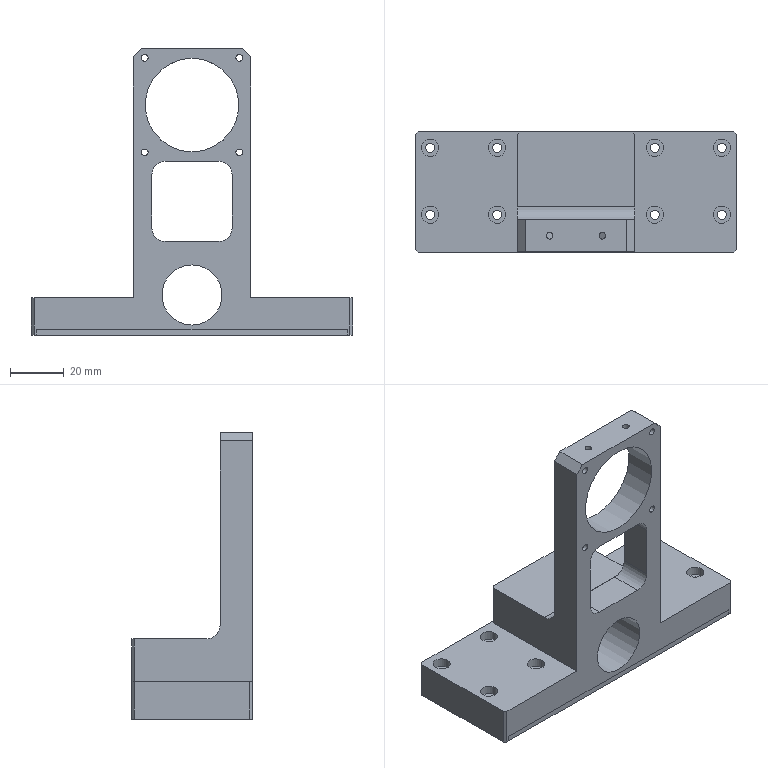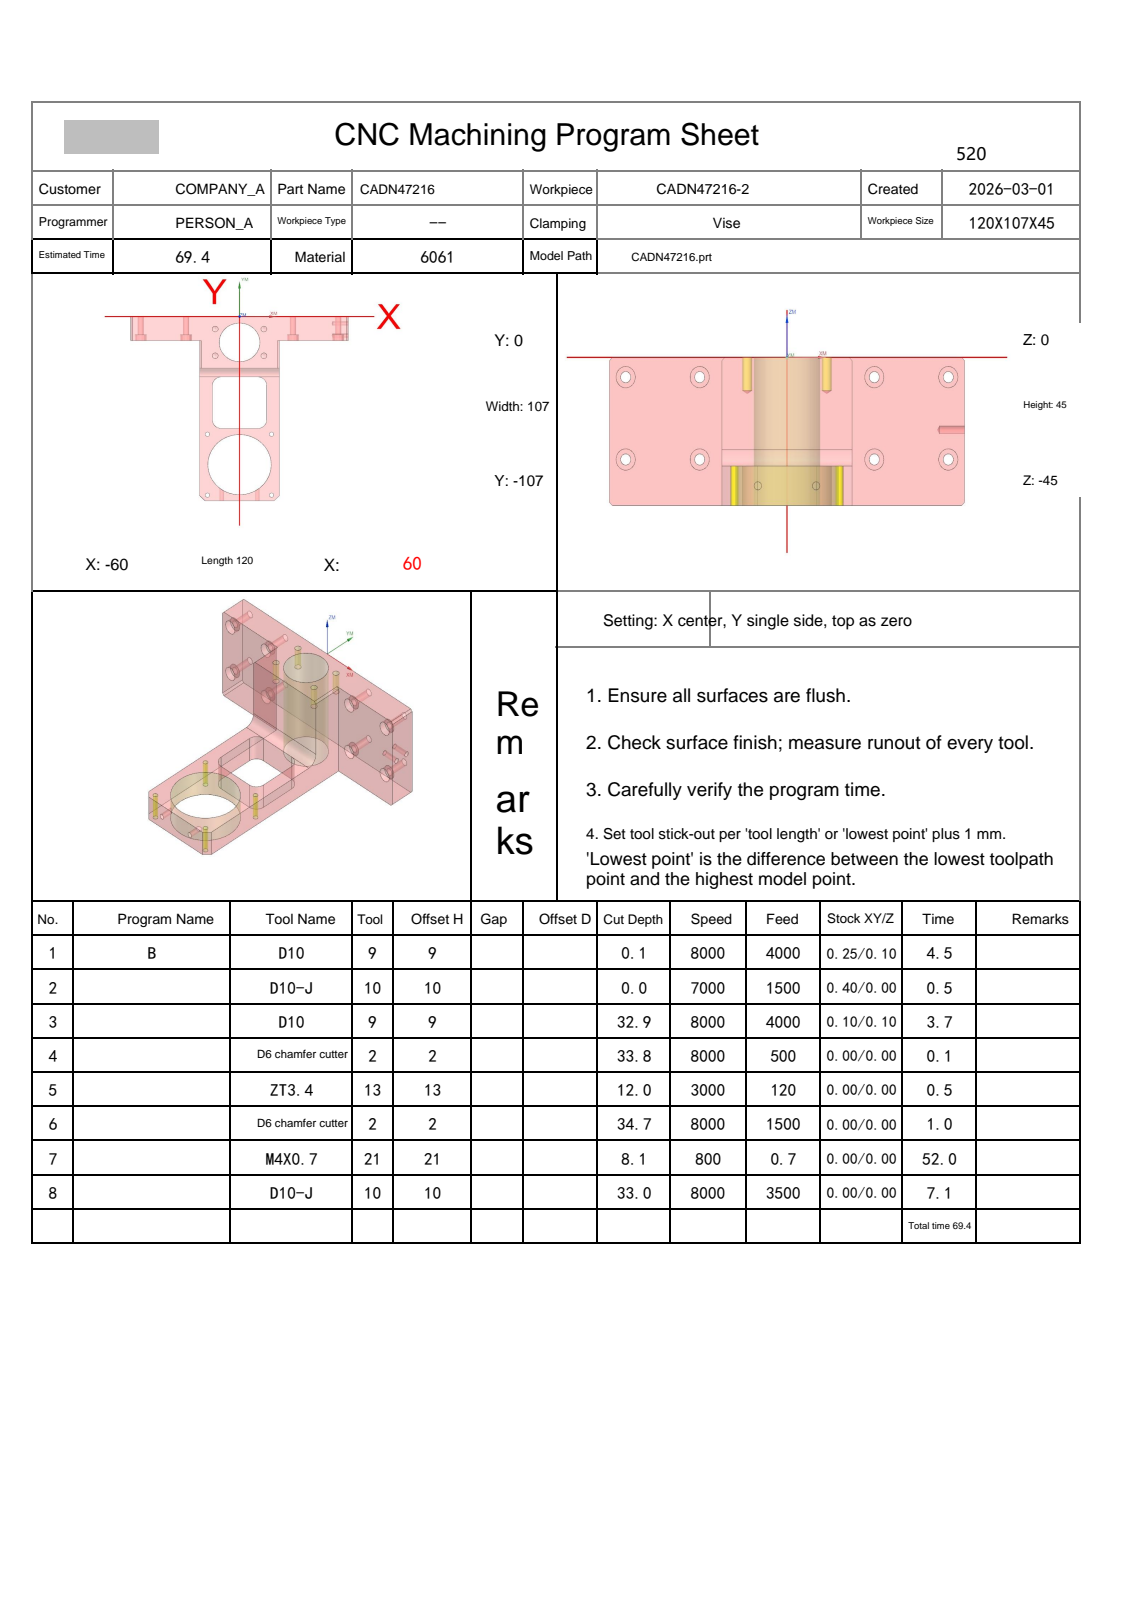NC program | NX | posted by the shop | part box 120 x 45 x 107 mm
Lines 4676 to 4990 of 8568:
N4 T02 M06
(D6 chamfer cutter  D=6. R=0. H=02 ce=0.00 di=0.10)
G00 G90 G54 X13.423 Y-22.75 M03 S8000
G43 H02 Z50.
M08
G98 G81 X13.423 Y-22.75 Z-.8 R1. F500.
Y-7.25
X-13.423
Y-22.75
X-17.678 Y-68.322 Z-33.8 R-32.
X17.678
Y-103.678
X-17.678
G80
G00 Z50.
G91 G28 Z0.0
M05
M09
G91 G28 Z0.0
M01
N5 T13 M06
(ZT3.4 D=3.4 DR_a=118 H=13)
G00 G90 G54 X13.423 Y-22.75 M03 S3000
G43 H13 Z50.
M08
G98 G83 X13.423 Y-22.75 Z-12. R1. F120. Q2.
Y-7.25
X-13.423
Y-22.75
G80
G00 Z50.
G91 G28 Z0.0
M05
M09
G91 G28 Z0.0
M01
N6 T02 M06
(D6 chamfer cutter  D=6. R=0. H=02 ce=0.00 di=0.10)
G00 G90 G54 X-17.678 Y-103.678 M03 S8000
G43 H02 Z50.
M08
G98 G81 X-17.678 Y-103.678 Z-34.75 R-30. F500.
X17.678
Y-68.322
X-17.678
G80
G00 Z50.
G00 G90 X13.423 Y-22.75 M03 S8000
Z50.
G98 G81 X13.423 Y-22.75 Z-2.2 R3. F500.
Y-7.25
X-13.423
Y-22.75
G80
G00 Z50.
G00 G90 X59.792 Y-14.99 M03 S6500
Z50.
Z.13
G01 Z-1.2 F1500.
G03 X59.452 Y-14.915 I-.601 J-1.907
G01 X59.398 Y-14.905
X59.349 Y-14.928
X59.259 Y-14.966
X59. Y-15.
X22.181
X22.175 Y-15.029
X22.172 Y-15.058
Z2.8
G00 Z10.
X21.792 Y-30.99
Z.13
G01 Z-1.2
G03 X21.452 Y-30.915 I-.601 J-1.907
G01 X21.398 Y-30.905
X21.349 Y-30.928
X21.259 Y-30.966
X21. Y-31.
X-21.
X-21.259 Y-30.966
X-21.349 Y-30.928
X-21.398 Y-30.905
X-21.452 Y-30.915
G03 X-21.792 Y-30.99 I.261 J-1.983
G01 Z.13
G00 Z10.
X-22.181 Y-15.
Z2.8
G01 Z-1.2
X-59.
X-59.259 Y-14.966
X-59.349 Y-14.928
X-59.398 Y-14.905
X-59.452 Y-14.915
G03 X-59.792 Y-14.99 I.261 J-1.983
G01 Z.13
G00 Z10.
Y.99
Z.13
G01 Z-1.2
G03 X-59.452 Y.915 I.601 J1.907
G01 X-59.398 Y.905
X-59.349 Y.928
X-59.259 Y.966
X-59. Y1.
X0.0
X59.
X59.259 Y.966
X59.349 Y.928
X59.398 Y.905
X59.452 Y.915
G03 X59.792 Y.99 I-.261 J1.983
G01 Z.13
G00 Z10.
X-13.842 Y-23.244
Z.405
G01 Z-1.2
G03 X-13.527 Y-23.391 I1. J1.732
G01 X-13.476 Y-23.412
X-13.423 Y-23.4
G03 X-12.773 Y-22.75 I0.0 J.65
X-13.423 Y-22.1 I-.65 J0.0
X-14.073 Y-22.75 I0.0 J-.65
X-13.423 Y-23.4 I.65 J0.0
G01 X-13.37 Y-23.412
X-13.32 Y-23.391
G03 X-13.004 Y-23.244 I-.684 J1.879
G01 Z.405
G00 Z10.
X-13.842 Y-7.744
Z.405
G01 Z-1.2
G03 X-13.527 Y-7.891 I1. J1.732
G01 X-13.476 Y-7.912
X-13.423 Y-7.9
G03 X-12.773 Y-7.25 I0.0 J.65
X-13.423 Y-6.6 I-.65 J0.0
X-14.073 Y-7.25 I0.0 J-.65
X-13.423 Y-7.9 I.65 J0.0
G01 X-13.37 Y-7.912
X-13.32 Y-7.891
G03 X-13.004 Y-7.744 I-.684 J1.879
G01 Z.405
G00 Z10.
X.395 Y-4.96
Z.207
G01 Z-1.2
G03 X.101 Y-4.772 I-1.218 J-1.587
G01 X.054 Y-4.745
X0.0 Y-4.75
G03 X-10.25 Y-15. I0.0 J-10.25
X0.0 Y-25.25 I10.25 J0.0
X10.25 Y-15. I0.0 J10.25
X0.0 Y-4.75 I-10.25 J0.0
G01 X-.054 Y-4.745
X-.101 Y-4.772
G03 X-.395 Y-4.96 I.923 J-1.774
G01 Z.207
G00 Z10.
X13.004 Y-23.244
Z.405
G01 Z-1.2
G03 X13.32 Y-23.391 I1. J1.732
G01 X13.37 Y-23.412
X13.423 Y-23.4
G03 X14.073 Y-22.75 I0.0 J.65
X13.423 Y-22.1 I-.65 J0.0
X12.773 Y-22.75 I0.0 J-.65
X13.423 Y-23.4 I.65 J0.0
G01 X13.476 Y-23.412
X13.527 Y-23.391
G03 X13.842 Y-23.244 I-.684 J1.879
G01 Z.405
G00 Z10.
X13.004 Y-7.744
Z.405
G01 Z-1.2
G03 X13.32 Y-7.891 I1. J1.732
G01 X13.37 Y-7.912
X13.423 Y-7.9
G03 X14.073 Y-7.25 I0.0 J.65
X13.423 Y-6.6 I-.65 J0.0
X12.773 Y-7.25 I0.0 J-.65
X13.423 Y-7.9 I.65 J0.0
G01 X13.476 Y-7.912
X13.527 Y-7.891
G03 X13.842 Y-7.744 I-.684 J1.879
G01 Z.405
G00 Z10.
X-9.651 Y-35.928
Z-30.199
G01 Z-34.199
X-9.741 Y-35.966
X-10. Y-36.
G03 X-14. Y-40. I0.0 J-4.
G01 Y-60.
G03 X-10. Y-64. I4. J0.0
G01 X10.
G03 X14. Y-60. I0.0 J4.
G01 Y-40.
G03 X10. Y-36. I-4. J0.0
G01 X9.946 Y-35.994
X9.898 Y-36.02
G03 X9.6 Y-36.201 I.885 J-1.794
G01 Z-32.802
G00 Z10.
X23.181 Y-34.692
Z-32.596
G01 Z-34.199
G03 X23.021 Y-34.92 I1.226 J-1.028
G01 X22.996 Y-34.956
X23. Y-35.
Y-104.
X22.966 Y-104.259
X22.866 Y-104.5
X22.707 Y-104.707
X19.707 Y-107.707
X19.5 Y-107.866
X19.259 Y-107.966
X19. Y-108.
X-19.
X-19.259 Y-107.966
X-19.5 Y-107.866
X-19.707 Y-107.707
X-22.707 Y-104.707
X-22.866 Y-104.5
X-22.966 Y-104.259
X-23. Y-104.
Y-35.
X-22.996 Y-34.956
X-23.021 Y-34.92
G03 X-23.181 Y-34.692 I-1.386 J-.8
G01 Z-32.596
G00 Z10.
X-.393 Y-102.286
Z-32.801
G01 Z-34.199
G03 X-.101 Y-102.476 I1.235 J1.573
G01 X-.054 Y-102.505
X0.0 Y-102.5
G03 X16.5 Y-86. I0.0 J16.5
X0.0 Y-69.5 I-16.5 J0.0
X-16.5 Y-86. I0.0 J-16.5
X0.0 Y-102.5 I16.5 J0.0
G01 X.054 Y-102.505
X.101 Y-102.476
G03 X.393 Y-102.286 I-.943 J1.764
G01 Z-32.801
G00 Z50.
G00 G90 X-60.708 Y-16.9 M03 S6500
Z50.
Z-.2
G01 Z-1.7 F1500.
X-60.699 Y-16.832
X-60.7 Y-16.763
Y2.763
X-60.699 Y2.832
X-60.708 Y2.9
Z-.2
G00 Z50.
X60.708
Z-.2
G01 Z-1.7
X60.699 Y2.832
X60.7 Y2.763
Y-16.763
X60.699 Y-16.832
X60.708 Y-16.9
Z-.2
G00 Z50.
G00 G90 X-23.227 Y-30.386 M03 S6500
Z50.
Z-.861
G01 Z-2. F1500.
G03 X-23.027 Y-30.1 I-1.532 J1.286
G01 X-22.997 Y-30.054
X-23. Y-30.
Y-16.
X-59.
G02 X-61. Y-14. I0.0 J2.
G01 Y0.0
G02 X-59. Y2. I2. J0.0
G01 X59.
G02 X61. Y0.0 I0.0 J-2.
G01 Y-14.
G02 X59. Y-16. I-2. J0.0
G01 X23.
Y-30.
X22.997 Y-30.054
X23.027 Y-30.1
G03 X23.227 Y-30.386 I1.732 J1.
G01 Z-.861
G00 Z50.
G91 G28 Z0.0
M05
M09
G91 G28 Z0.0
M01
N7 T21 M06
(M4X0.7 D=3.3 DR_a=180 H=21)
G00 G90 G54 X13.423 Y-22.75 M03 S800
G43 H21 Z50.
M08
G95
G98 G84 X13.423 Y-22.75 Z-8.1 R1. F.7 Q3.
Y-7.25
X-13.423
Y-22.75
G80
G94
G00 Z50.
G91 G28 Z0.0
M05
M09
G91 G28 Z0.0
M01